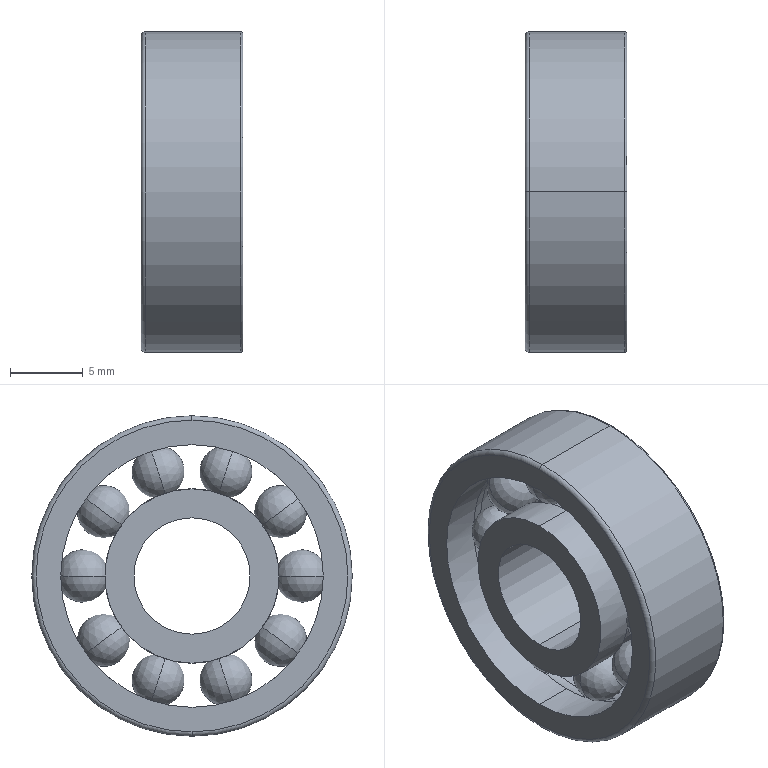Part | NX | features BREP 1 | 1 solid | 75 faces | box 7 x 22 x 22 mm | volume 1425 mm3 | torus 39 | sphere 20 | cylinder 10 | plane 4 | cone 2 | commonest cylinder face diameters 11.969 x4 8 x2 18.031 x2 22 x2